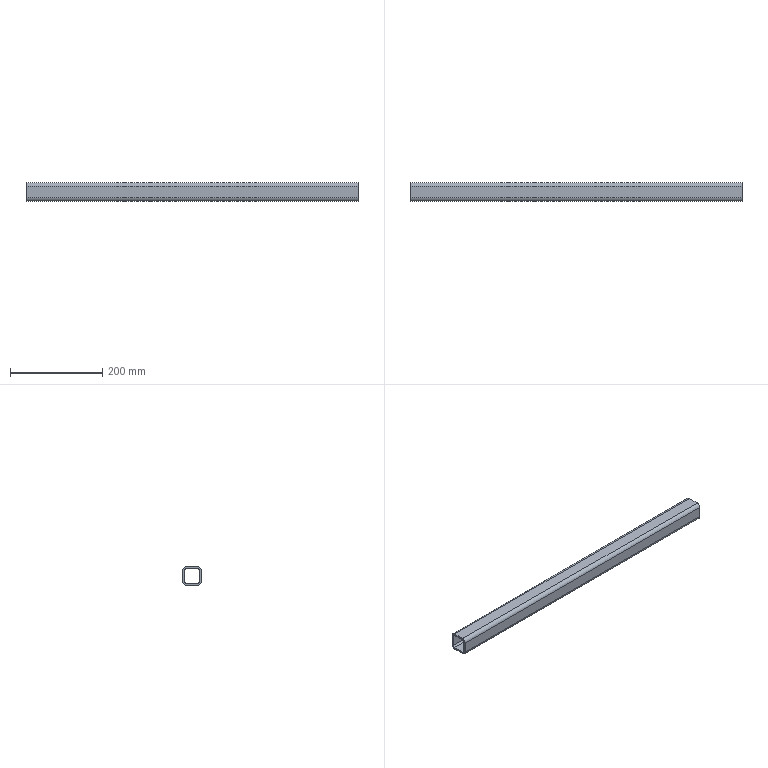Part | SolidWorks | features WeldMemberFeat 1, WeldmentFeature 1 | 1 solid | 18 faces | box 720 x 40 x 40 mm | volume 385053 mm3 | plane 10 | cylinder 8 | commonest cylinder face diameters 8 x4 16 x4
STEP:
#1=CARTESIAN_POINT('',(-1000.,20.,12.));
#2=VERTEX_POINT('',#1);
#3=CARTESIAN_POINT('',(-1000.,12.,20.));
#4=VERTEX_POINT('',#3);
#5=CARTESIAN_POINT('',(-1000.,12.,12.));
#6=DIRECTION('',(1.,0.,0.));
#7=DIRECTION('',(0.,0.,-1.));
#8=AXIS2_PLACEMENT_3D('',#5,#6,#7);
#9=CIRCLE('',#8,8.);
#10=EDGE_CURVE('',#2,#4,#9,.T.);
#11=ORIENTED_EDGE('',*,*,#10,.T.);
#12=CARTESIAN_POINT('',(-280.,12.,20.));
#13=VERTEX_POINT('',#12);
#14=CARTESIAN_POINT('',(-280.,12.,20.));
#15=DIRECTION('',(-1.,0.,0.));
#16=VECTOR('',#15,1000.);
#17=LINE('',#14,#16);
#18=EDGE_CURVE('',#13,#4,#17,.T.);
#19=ORIENTED_EDGE('',*,*,#18,.F.);
#20=CARTESIAN_POINT('',(-280.,20.,12.));
#21=VERTEX_POINT('',#20);
#22=CARTESIAN_POINT('',(-280.,12.,12.));
#23=DIRECTION('',(1.,0.,0.));
#24=DIRECTION('',(0.,0.,-1.));
#25=AXIS2_PLACEMENT_3D('',#22,#23,#24);
#26=CIRCLE('',#25,8.);
#27=EDGE_CURVE('',#21,#13,#26,.T.);
#28=ORIENTED_EDGE('',*,*,#27,.F.);
#29=CARTESIAN_POINT('',(-280.,20.,12.));
#30=DIRECTION('',(-1.,0.,0.));
#31=VECTOR('',#30,1000.);
#32=LINE('',#29,#31);
#33=EDGE_CURVE('',#21,#2,#32,.T.);
#34=ORIENTED_EDGE('',*,*,#33,.T.);
#35=EDGE_LOOP('',(#11,#19,#28,#34));
#36=FACE_OUTER_BOUND('',#35,.T.);
#37=CARTESIAN_POINT('',(-280.,12.,12.));
#38=DIRECTION('',(-1.,0.,0.));
#39=DIRECTION('',(0.,0.,1.));
#40=AXIS2_PLACEMENT_3D('',#37,#38,#39);
#41=CYLINDRICAL_SURFACE('',#40,8.);
#42=ADVANCED_FACE('',(#36),#41,.T.);
#43=CARTESIAN_POINT('',(-1000.,-12.,20.));
#44=VERTEX_POINT('',#43);
#45=CARTESIAN_POINT('',(-1000.,12.,20.));
#46=DIRECTION('',(0.,-1.,0.));
#47=VECTOR('',#46,1000.);
#48=LINE('',#45,#47);
#49=EDGE_CURVE('',#4,#44,#48,.T.);
#50=ORIENTED_EDGE('',*,*,#49,.T.);
#51=CARTESIAN_POINT('',(-280.,-12.,20.));
#52=VERTEX_POINT('',#51);
#53=CARTESIAN_POINT('',(-280.,-12.,20.));
#54=DIRECTION('',(-1.,0.,0.));
#55=VECTOR('',#54,1000.);
#56=LINE('',#53,#55);
#57=EDGE_CURVE('',#52,#44,#56,.T.);
#58=ORIENTED_EDGE('',*,*,#57,.F.);
#59=CARTESIAN_POINT('',(-280.,12.,20.));
#60=DIRECTION('',(0.,-1.,0.));
#61=VECTOR('',#60,1000.);
#62=LINE('',#59,#61);
#63=EDGE_CURVE('',#13,#52,#62,.T.);
#64=ORIENTED_EDGE('',*,*,#63,.F.);
#65=ORIENTED_EDGE('',*,*,#18,.T.);
#66=EDGE_LOOP('',(#50,#58,#64,#65));
#67=FACE_OUTER_BOUND('',#66,.T.);
#68=CARTESIAN_POINT('',(-280.,12.,20.));
#69=DIRECTION('',(0.,0.,-1.));
#70=DIRECTION('',(-1.,0.,0.));
#71=AXIS2_PLACEMENT_3D('',#68,#69,#70);
#72=PLANE('',#71);
#73=ADVANCED_FACE('',(#67),#72,.F.);
#74=CARTESIAN_POINT('',(-1000.,-20.,12.));
#75=VERTEX_POINT('',#74);
#76=CARTESIAN_POINT('',(-1000.,-12.,12.));
#77=DIRECTION('',(1.,0.,0.));
#78=DIRECTION('',(0.,0.,-1.));
#79=AXIS2_PLACEMENT_3D('',#76,#77,#78);
#80=CIRCLE('',#79,8.);
#81=EDGE_CURVE('',#44,#75,#80,.T.);
#82=ORIENTED_EDGE('',*,*,#81,.T.);
#83=CARTESIAN_POINT('',(-280.,-20.,12.));
#84=VERTEX_POINT('',#83);
#85=CARTESIAN_POINT('',(-280.,-20.,12.));
#86=DIRECTION('',(-1.,0.,0.));
#87=VECTOR('',#86,1000.);
#88=LINE('',#85,#87);
#89=EDGE_CURVE('',#84,#75,#88,.T.);
#90=ORIENTED_EDGE('',*,*,#89,.F.);
#91=CARTESIAN_POINT('',(-280.,-12.,12.));
#92=DIRECTION('',(1.,0.,0.));
#93=DIRECTION('',(0.,0.,-1.));
#94=AXIS2_PLACEMENT_3D('',#91,#92,#93);
#95=CIRCLE('',#94,8.);
#96=EDGE_CURVE('',#52,#84,#95,.T.);
#97=ORIENTED_EDGE('',*,*,#96,.F.);
#98=ORIENTED_EDGE('',*,*,#57,.T.);
#99=EDGE_LOOP('',(#82,#90,#97,#98));
#100=FACE_OUTER_BOUND('',#99,.T.);
#101=CARTESIAN_POINT('',(-280.,-12.,12.));
#102=DIRECTION('',(-1.,0.,0.));
#103=DIRECTION('',(0.,0.,1.));
#104=AXIS2_PLACEMENT_3D('',#101,#102,#103);
#105=CYLINDRICAL_SURFACE('',#104,8.);
#106=ADVANCED_FACE('',(#100),#105,.T.);
#107=CARTESIAN_POINT('',(-1000.,-20.,-12.));
#108=VERTEX_POINT('',#107);
#109=CARTESIAN_POINT('',(-1000.,-20.,-12.));
#110=DIRECTION('',(0.,0.,-1.));
#111=VECTOR('',#110,1000.);
#112=LINE('',#109,#111);
#113=EDGE_CURVE('',#75,#108,#112,.T.);
#114=ORIENTED_EDGE('',*,*,#113,.T.);
#115=CARTESIAN_POINT('',(-280.,-20.,-12.));
#116=VERTEX_POINT('',#115);
#117=CARTESIAN_POINT('',(-280.,-20.,-12.));
#118=DIRECTION('',(-1.,0.,0.));
#119=VECTOR('',#118,1000.);
#120=LINE('',#117,#119);
#121=EDGE_CURVE('',#116,#108,#120,.T.);
#122=ORIENTED_EDGE('',*,*,#121,.F.);
#123=CARTESIAN_POINT('',(-280.,-20.,-12.));
#124=DIRECTION('',(0.,0.,-1.));
#125=VECTOR('',#124,1000.);
#126=LINE('',#123,#125);
#127=EDGE_CURVE('',#84,#116,#126,.T.);
#128=ORIENTED_EDGE('',*,*,#127,.F.);
#129=ORIENTED_EDGE('',*,*,#89,.T.);
#130=EDGE_LOOP('',(#114,#122,#128,#129));
#131=FACE_OUTER_BOUND('',#130,.T.);
#132=CARTESIAN_POINT('',(-280.,-20.,-12.));
#133=DIRECTION('',(0.,1.,0.));
#134=DIRECTION('',(0.,0.,1.));
#135=AXIS2_PLACEMENT_3D('',#132,#133,#134);
#136=PLANE('',#135);
#137=ADVANCED_FACE('',(#131),#136,.F.);
#138=CARTESIAN_POINT('',(-1000.,-12.,-20.));
#139=VERTEX_POINT('',#138);
#140=CARTESIAN_POINT('',(-1000.,-12.,-12.));
#141=DIRECTION('',(1.,0.,0.));
#142=DIRECTION('',(0.,0.,-1.));
#143=AXIS2_PLACEMENT_3D('',#140,#141,#142);
#144=CIRCLE('',#143,8.);
#145=EDGE_CURVE('',#108,#139,#144,.T.);
#146=ORIENTED_EDGE('',*,*,#145,.T.);
#147=CARTESIAN_POINT('',(-280.,-12.,-20.));
#148=VERTEX_POINT('',#147);
#149=CARTESIAN_POINT('',(-280.,-12.,-20.));
#150=DIRECTION('',(-1.,0.,0.));
#151=VECTOR('',#150,1000.);
#152=LINE('',#149,#151);
#153=EDGE_CURVE('',#148,#139,#152,.T.);
#154=ORIENTED_EDGE('',*,*,#153,.F.);
#155=CARTESIAN_POINT('',(-280.,-12.,-12.));
#156=DIRECTION('',(1.,0.,0.));
#157=DIRECTION('',(0.,0.,-1.));
#158=AXIS2_PLACEMENT_3D('',#155,#156,#157);
#159=CIRCLE('',#158,8.);
#160=EDGE_CURVE('',#116,#148,#159,.T.);
#161=ORIENTED_EDGE('',*,*,#160,.F.);
#162=ORIENTED_EDGE('',*,*,#121,.T.);
#163=EDGE_LOOP('',(#146,#154,#161,#162));
#164=FACE_OUTER_BOUND('',#163,.T.);
#165=CARTESIAN_POINT('',(-280.,-12.,-12.));
#166=DIRECTION('',(-1.,0.,0.));
#167=DIRECTION('',(0.,0.,1.));
#168=AXIS2_PLACEMENT_3D('',#165,#166,#167);
#169=CYLINDRICAL_SURFACE('',#168,8.);
#170=ADVANCED_FACE('',(#164),#169,.T.);
#171=CARTESIAN_POINT('',(-1000.,12.,-20.));
#172=VERTEX_POINT('',#171);
#173=CARTESIAN_POINT('',(-1000.,-12.,-20.));
#174=DIRECTION('',(0.,1.,0.));
#175=VECTOR('',#174,1000.);
#176=LINE('',#173,#175);
#177=EDGE_CURVE('',#139,#172,#176,.T.);
#178=ORIENTED_EDGE('',*,*,#177,.T.);
#179=CARTESIAN_POINT('',(-280.,12.,-20.));
#180=VERTEX_POINT('',#179);
#181=CARTESIAN_POINT('',(-280.,12.,-20.));
#182=DIRECTION('',(-1.,0.,0.));
#183=VECTOR('',#182,1000.);
#184=LINE('',#181,#183);
#185=EDGE_CURVE('',#180,#172,#184,.T.);
#186=ORIENTED_EDGE('',*,*,#185,.F.);
#187=CARTESIAN_POINT('',(-280.,-12.,-20.));
#188=DIRECTION('',(0.,1.,0.));
#189=VECTOR('',#188,1000.);
#190=LINE('',#187,#189);
#191=EDGE_CURVE('',#148,#180,#190,.T.);
#192=ORIENTED_EDGE('',*,*,#191,.F.);
#193=ORIENTED_EDGE('',*,*,#153,.T.);
#194=EDGE_LOOP('',(#178,#186,#192,#193));
#195=FACE_OUTER_BOUND('',#194,.T.);
#196=CARTESIAN_POINT('',(-280.,-12.,-20.));
#197=DIRECTION('',(0.,0.,1.));
#198=DIRECTION('',(1.,0.,0.));
#199=AXIS2_PLACEMENT_3D('',#196,#197,#198);
#200=PLANE('',#199);
#201=ADVANCED_FACE('',(#195),#200,.F.);
#202=CARTESIAN_POINT('',(-1000.,20.,-12.));
#203=VERTEX_POINT('',#202);
#204=CARTESIAN_POINT('',(-1000.,12.,-12.));
#205=DIRECTION('',(1.,0.,0.));
#206=DIRECTION('',(0.,0.,-1.));
#207=AXIS2_PLACEMENT_3D('',#204,#205,#206);
#208=CIRCLE('',#207,8.);
#209=EDGE_CURVE('',#172,#203,#208,.T.);
#210=ORIENTED_EDGE('',*,*,#209,.T.);
#211=CARTESIAN_POINT('',(-280.,20.,-12.));
#212=VERTEX_POINT('',#211);
#213=CARTESIAN_POINT('',(-280.,20.,-12.));
#214=DIRECTION('',(-1.,0.,0.));
#215=VECTOR('',#214,1000.);
#216=LINE('',#213,#215);
#217=EDGE_CURVE('',#212,#203,#216,.T.);
#218=ORIENTED_EDGE('',*,*,#217,.F.);
#219=CARTESIAN_POINT('',(-280.,12.,-12.));
#220=DIRECTION('',(1.,0.,0.));
#221=DIRECTION('',(0.,0.,-1.));
#222=AXIS2_PLACEMENT_3D('',#219,#220,#221);
#223=CIRCLE('',#222,8.);
#224=EDGE_CURVE('',#180,#212,#223,.T.);
#225=ORIENTED_EDGE('',*,*,#224,.F.);
#226=ORIENTED_EDGE('',*,*,#185,.T.);
#227=EDGE_LOOP('',(#210,#218,#225,#226));
#228=FACE_OUTER_BOUND('',#227,.T.);
#229=CARTESIAN_POINT('',(-280.,12.,-12.));
#230=DIRECTION('',(-1.,0.,0.));
#231=DIRECTION('',(0.,0.,1.));
#232=AXIS2_PLACEMENT_3D('',#229,#230,#231);
#233=CYLINDRICAL_SURFACE('',#232,8.);
#234=ADVANCED_FACE('',(#228),#233,.T.);
#235=CARTESIAN_POINT('',(-1000.,-12.,16.));
#236=VERTEX_POINT('',#235);
#237=CARTESIAN_POINT('',(-1000.,-16.,12.));
#238=VERTEX_POINT('',#237);
#239=CARTESIAN_POINT('',(-1000.,-12.,12.));
#240=DIRECTION('',(1.,0.,0.));
#241=DIRECTION('',(0.,0.,-1.));
#242=AXIS2_PLACEMENT_3D('',#239,#240,#241);
#243=CIRCLE('',#242,4.);
#244=EDGE_CURVE('',#236,#238,#243,.T.);
#245=ORIENTED_EDGE('',*,*,#244,.F.);
#246=CARTESIAN_POINT('',(-280.,-12.,16.));
#247=VERTEX_POINT('',#246);
#248=CARTESIAN_POINT('',(-280.,-12.,16.));
#249=DIRECTION('',(-1.,0.,0.));
#250=VECTOR('',#249,1000.);
#251=LINE('',#248,#250);
#252=EDGE_CURVE('',#247,#236,#251,.T.);
#253=ORIENTED_EDGE('',*,*,#252,.F.);
#254=CARTESIAN_POINT('',(-280.,-16.,12.));
#255=VERTEX_POINT('',#254);
#256=CARTESIAN_POINT('',(-280.,-12.,12.));
#257=DIRECTION('',(1.,0.,0.));
#258=DIRECTION('',(0.,0.,-1.));
#259=AXIS2_PLACEMENT_3D('',#256,#257,#258);
#260=CIRCLE('',#259,4.);
#261=EDGE_CURVE('',#247,#255,#260,.T.);
#262=ORIENTED_EDGE('',*,*,#261,.T.);
#263=CARTESIAN_POINT('',(-280.,-16.,12.));
#264=DIRECTION('',(-1.,0.,0.));
#265=VECTOR('',#264,1000.);
#266=LINE('',#263,#265);
#267=EDGE_CURVE('',#255,#238,#266,.T.);
#268=ORIENTED_EDGE('',*,*,#267,.T.);
#269=EDGE_LOOP('',(#245,#253,#262,#268));
#270=FACE_OUTER_BOUND('',#269,.T.);
#271=CARTESIAN_POINT('',(-280.,-12.,12.));
#272=DIRECTION('',(-1.,0.,0.));
#273=DIRECTION('',(0.,0.,1.));
#274=AXIS2_PLACEMENT_3D('',#271,#272,#273);
#275=CYLINDRICAL_SURFACE('',#274,4.);
#276=ADVANCED_FACE('',(#270),#275,.F.);
#277=CARTESIAN_POINT('',(-1000.,12.,16.));
#278=VERTEX_POINT('',#277);
#279=CARTESIAN_POINT('',(-1000.,12.,16.));
#280=DIRECTION('',(0.,-1.,0.));
#281=VECTOR('',#280,1000.);
#282=LINE('',#279,#281);
#283=EDGE_CURVE('',#278,#236,#282,.T.);
#284=ORIENTED_EDGE('',*,*,#283,.F.);
#285=CARTESIAN_POINT('',(-280.,12.,16.));
#286=VERTEX_POINT('',#285);
#287=CARTESIAN_POINT('',(-280.,12.,16.));
#288=DIRECTION('',(-1.,0.,0.));
#289=VECTOR('',#288,1000.);
#290=LINE('',#287,#289);
#291=EDGE_CURVE('',#286,#278,#290,.T.);
#292=ORIENTED_EDGE('',*,*,#291,.F.);
#293=CARTESIAN_POINT('',(-280.,12.,16.));
#294=DIRECTION('',(0.,-1.,0.));
#295=VECTOR('',#294,1000.);
#296=LINE('',#293,#295);
#297=EDGE_CURVE('',#286,#247,#296,.T.);
#298=ORIENTED_EDGE('',*,*,#297,.T.);
#299=ORIENTED_EDGE('',*,*,#252,.T.);
#300=EDGE_LOOP('',(#284,#292,#298,#299));
#301=FACE_OUTER_BOUND('',#300,.T.);
#302=CARTESIAN_POINT('',(-280.,12.,16.));
#303=DIRECTION('',(0.,0.,-1.));
#304=DIRECTION('',(-1.,0.,0.));
#305=AXIS2_PLACEMENT_3D('',#302,#303,#304);
#306=PLANE('',#305);
#307=ADVANCED_FACE('',(#301),#306,.T.);
#308=CARTESIAN_POINT('',(-1000.,16.,12.));
#309=VERTEX_POINT('',#308);
#310=CARTESIAN_POINT('',(-1000.,12.,12.));
#311=DIRECTION('',(1.,0.,0.));
#312=DIRECTION('',(0.,0.,-1.));
#313=AXIS2_PLACEMENT_3D('',#310,#311,#312);
#314=CIRCLE('',#313,4.);
#315=EDGE_CURVE('',#309,#278,#314,.T.);
#316=ORIENTED_EDGE('',*,*,#315,.F.);
#317=CARTESIAN_POINT('',(-280.,16.,12.));
#318=VERTEX_POINT('',#317);
#319=CARTESIAN_POINT('',(-280.,16.,12.));
#320=DIRECTION('',(-1.,0.,0.));
#321=VECTOR('',#320,1000.);
#322=LINE('',#319,#321);
#323=EDGE_CURVE('',#318,#309,#322,.T.);
#324=ORIENTED_EDGE('',*,*,#323,.F.);
#325=CARTESIAN_POINT('',(-280.,12.,12.));
#326=DIRECTION('',(1.,0.,0.));
#327=DIRECTION('',(0.,0.,-1.));
#328=AXIS2_PLACEMENT_3D('',#325,#326,#327);
#329=CIRCLE('',#328,4.);
#330=EDGE_CURVE('',#318,#286,#329,.T.);
#331=ORIENTED_EDGE('',*,*,#330,.T.);
#332=ORIENTED_EDGE('',*,*,#291,.T.);
#333=EDGE_LOOP('',(#316,#324,#331,#332));
#334=FACE_OUTER_BOUND('',#333,.T.);
#335=CARTESIAN_POINT('',(-280.,12.,12.));
#336=DIRECTION('',(-1.,0.,0.));
#337=DIRECTION('',(0.,0.,1.));
#338=AXIS2_PLACEMENT_3D('',#335,#336,#337);
#339=CYLINDRICAL_SURFACE('',#338,4.);
#340=ADVANCED_FACE('',(#334),#339,.F.);
#341=CARTESIAN_POINT('',(-1000.,16.,-12.));
#342=VERTEX_POINT('',#341);
#343=CARTESIAN_POINT('',(-1000.,16.,12.));
#344=DIRECTION('',(0.,0.,1.));
#345=VECTOR('',#344,1000.);
#346=LINE('',#343,#345);
#347=EDGE_CURVE('',#342,#309,#346,.T.);
#348=ORIENTED_EDGE('',*,*,#347,.F.);
#349=CARTESIAN_POINT('',(-280.,16.,-12.));
#350=VERTEX_POINT('',#349);
#351=CARTESIAN_POINT('',(-280.,16.,-12.));
#352=DIRECTION('',(-1.,0.,0.));
#353=VECTOR('',#352,1000.);
#354=LINE('',#351,#353);
#355=EDGE_CURVE('',#350,#342,#354,.T.);
#356=ORIENTED_EDGE('',*,*,#355,.F.);
#357=CARTESIAN_POINT('',(-280.,16.,12.));
#358=DIRECTION('',(0.,0.,1.));
#359=VECTOR('',#358,1000.);
#360=LINE('',#357,#359);
#361=EDGE_CURVE('',#350,#318,#360,.T.);
#362=ORIENTED_EDGE('',*,*,#361,.T.);
#363=ORIENTED_EDGE('',*,*,#323,.T.);
#364=EDGE_LOOP('',(#348,#356,#362,#363));
#365=FACE_OUTER_BOUND('',#364,.T.);
#366=CARTESIAN_POINT('',(-280.,16.,12.));
#367=DIRECTION('',(0.,-1.,0.));
#368=DIRECTION('',(0.,0.,-1.));
#369=AXIS2_PLACEMENT_3D('',#366,#367,#368);
#370=PLANE('',#369);
#371=ADVANCED_FACE('',(#365),#370,.T.);
#372=CARTESIAN_POINT('',(-1000.,12.,-16.));
#373=VERTEX_POINT('',#372);
#374=CARTESIAN_POINT('',(-1000.,12.,-12.));
#375=DIRECTION('',(1.,0.,0.));
#376=DIRECTION('',(0.,0.,-1.));
#377=AXIS2_PLACEMENT_3D('',#374,#375,#376);
#378=CIRCLE('',#377,4.);
#379=EDGE_CURVE('',#373,#342,#378,.T.);
#380=ORIENTED_EDGE('',*,*,#379,.F.);
#381=CARTESIAN_POINT('',(-280.,12.,-16.));
#382=VERTEX_POINT('',#381);
#383=CARTESIAN_POINT('',(-280.,12.,-16.));
#384=DIRECTION('',(-1.,0.,0.));
#385=VECTOR('',#384,1000.);
#386=LINE('',#383,#385);
#387=EDGE_CURVE('',#382,#373,#386,.T.);
#388=ORIENTED_EDGE('',*,*,#387,.F.);
#389=CARTESIAN_POINT('',(-280.,12.,-12.));
#390=DIRECTION('',(1.,0.,0.));
#391=DIRECTION('',(0.,0.,-1.));
#392=AXIS2_PLACEMENT_3D('',#389,#390,#391);
#393=CIRCLE('',#392,4.);
#394=EDGE_CURVE('',#382,#350,#393,.T.);
#395=ORIENTED_EDGE('',*,*,#394,.T.);
#396=ORIENTED_EDGE('',*,*,#355,.T.);
#397=EDGE_LOOP('',(#380,#388,#395,#396));
#398=FACE_OUTER_BOUND('',#397,.T.);
#399=CARTESIAN_POINT('',(-280.,12.,-12.));
#400=DIRECTION('',(-1.,0.,0.));
#401=DIRECTION('',(0.,0.,1.));
#402=AXIS2_PLACEMENT_3D('',#399,#400,#401);
#403=CYLINDRICAL_SURFACE('',#402,4.);
#404=ADVANCED_FACE('',(#398),#403,.F.);
#405=CARTESIAN_POINT('',(-1000.,-12.,-16.));
#406=VERTEX_POINT('',#405);
#407=CARTESIAN_POINT('',(-1000.,-12.,-16.));
#408=DIRECTION('',(0.,1.,0.));
#409=VECTOR('',#408,1000.);
#410=LINE('',#407,#409);
#411=EDGE_CURVE('',#406,#373,#410,.T.);
#412=ORIENTED_EDGE('',*,*,#411,.F.);
#413=CARTESIAN_POINT('',(-280.,-12.,-16.));
#414=VERTEX_POINT('',#413);
#415=CARTESIAN_POINT('',(-280.,-12.,-16.));
#416=DIRECTION('',(-1.,0.,0.));
#417=VECTOR('',#416,1000.);
#418=LINE('',#415,#417);
#419=EDGE_CURVE('',#414,#406,#418,.T.);
#420=ORIENTED_EDGE('',*,*,#419,.F.);
#421=CARTESIAN_POINT('',(-280.,-12.,-16.));
#422=DIRECTION('',(0.,1.,0.));
#423=VECTOR('',#422,1000.);
#424=LINE('',#421,#423);
#425=EDGE_CURVE('',#414,#382,#424,.T.);
#426=ORIENTED_EDGE('',*,*,#425,.T.);
#427=ORIENTED_EDGE('',*,*,#387,.T.);
#428=EDGE_LOOP('',(#412,#420,#426,#427));
#429=FACE_OUTER_BOUND('',#428,.T.);
#430=CARTESIAN_POINT('',(-280.,-12.,-16.));
#431=DIRECTION('',(0.,0.,1.));
#432=DIRECTION('',(1.,0.,0.));
#433=AXIS2_PLACEMENT_3D('',#430,#431,#432);
#434=PLANE('',#433);
#435=ADVANCED_FACE('',(#429),#434,.T.);
#436=CARTESIAN_POINT('',(-1000.,-16.,-12.));
#437=VERTEX_POINT('',#436);
#438=CARTESIAN_POINT('',(-1000.,-12.,-12.));
#439=DIRECTION('',(1.,0.,0.));
#440=DIRECTION('',(0.,0.,-1.));
#441=AXIS2_PLACEMENT_3D('',#438,#439,#440);
#442=CIRCLE('',#441,4.);
#443=EDGE_CURVE('',#437,#406,#442,.T.);
#444=ORIENTED_EDGE('',*,*,#443,.F.);
#445=CARTESIAN_POINT('',(-280.,-16.,-12.));
#446=VERTEX_POINT('',#445);
#447=CARTESIAN_POINT('',(-280.,-16.,-12.));
#448=DIRECTION('',(-1.,0.,0.));
#449=VECTOR('',#448,1000.);
#450=LINE('',#447,#449);
#451=EDGE_CURVE('',#446,#437,#450,.T.);
#452=ORIENTED_EDGE('',*,*,#451,.F.);
#453=CARTESIAN_POINT('',(-280.,-12.,-12.));
#454=DIRECTION('',(1.,0.,0.));
#455=DIRECTION('',(0.,0.,-1.));
#456=AXIS2_PLACEMENT_3D('',#453,#454,#455);
#457=CIRCLE('',#456,4.);
#458=EDGE_CURVE('',#446,#414,#457,.T.);
#459=ORIENTED_EDGE('',*,*,#458,.T.);
#460=ORIENTED_EDGE('',*,*,#419,.T.);
#461=EDGE_LOOP('',(#444,#452,#459,#460));
#462=FACE_OUTER_BOUND('',#461,.T.);
#463=CARTESIAN_POINT('',(-280.,-12.,-12.));
#464=DIRECTION('',(-1.,0.,0.));
#465=DIRECTION('',(0.,0.,1.));
#466=AXIS2_PLACEMENT_3D('',#463,#464,#465);
#467=CYLINDRICAL_SURFACE('',#466,4.);
#468=ADVANCED_FACE('',(#462),#467,.F.);
#469=CARTESIAN_POINT('',(-1000.,-16.,-12.));
#470=DIRECTION('',(0.,0.,-1.));
#471=VECTOR('',#470,1000.);
#472=LINE('',#469,#471);
#473=EDGE_CURVE('',#238,#437,#472,.T.);
#474=ORIENTED_EDGE('',*,*,#473,.F.);
#475=ORIENTED_EDGE('',*,*,#267,.F.);
#476=CARTESIAN_POINT('',(-280.,-16.,-12.));
#477=DIRECTION('',(0.,0.,-1.));
#478=VECTOR('',#477,1000.);
#479=LINE('',#476,#478);
#480=EDGE_CURVE('',#255,#446,#479,.T.);
#481=ORIENTED_EDGE('',*,*,#480,.T.);
#482=ORIENTED_EDGE('',*,*,#451,.T.);
#483=EDGE_LOOP('',(#474,#475,#481,#482));
#484=FACE_OUTER_BOUND('',#483,.T.);
#485=CARTESIAN_POINT('',(-280.,-16.,-12.));
#486=DIRECTION('',(0.,1.,0.));
#487=DIRECTION('',(0.,0.,1.));
#488=AXIS2_PLACEMENT_3D('',#485,#486,#487);
#489=PLANE('',#488);
#490=ADVANCED_FACE('',(#484),#489,.T.);
#491=CARTESIAN_POINT('',(-1000.,20.,12.));
#492=DIRECTION('',(0.,0.,1.));
#493=VECTOR('',#492,1000.);
#494=LINE('',#491,#493);
#495=EDGE_CURVE('',#203,#2,#494,.T.);
#496=ORIENTED_EDGE('',*,*,#495,.T.);
#497=ORIENTED_EDGE('',*,*,#33,.F.);
#498=CARTESIAN_POINT('',(-280.,20.,12.));
#499=DIRECTION('',(0.,0.,1.));
#500=VECTOR('',#499,1000.);
#501=LINE('',#498,#500);
#502=EDGE_CURVE('',#212,#21,#501,.T.);
#503=ORIENTED_EDGE('',*,*,#502,.F.);
#504=ORIENTED_EDGE('',*,*,#217,.T.);
#505=EDGE_LOOP('',(#496,#497,#503,#504));
#506=FACE_OUTER_BOUND('',#505,.T.);
#507=CARTESIAN_POINT('',(-280.,20.,12.));
#508=DIRECTION('',(0.,-1.,0.));
#509=DIRECTION('',(0.,0.,-1.));
#510=AXIS2_PLACEMENT_3D('',#507,#508,#509);
#511=PLANE('',#510);
#512=ADVANCED_FACE('',(#506),#511,.F.);
#513=ORIENTED_EDGE('',*,*,#261,.F.);
#514=ORIENTED_EDGE('',*,*,#297,.F.);
#515=ORIENTED_EDGE('',*,*,#330,.F.);
#516=ORIENTED_EDGE('',*,*,#361,.F.);
#517=ORIENTED_EDGE('',*,*,#394,.F.);
#518=ORIENTED_EDGE('',*,*,#425,.F.);
#519=ORIENTED_EDGE('',*,*,#458,.F.);
#520=ORIENTED_EDGE('',*,*,#480,.F.);
#521=EDGE_LOOP('',(#513,#514,#515,#516,#517,#518,#519,#520));
#522=FACE_BOUND('',#521,.T.);
#523=ORIENTED_EDGE('',*,*,#27,.T.);
#524=ORIENTED_EDGE('',*,*,#63,.T.);
#525=ORIENTED_EDGE('',*,*,#96,.T.);
#526=ORIENTED_EDGE('',*,*,#127,.T.);
#527=ORIENTED_EDGE('',*,*,#160,.T.);
#528=ORIENTED_EDGE('',*,*,#191,.T.);
#529=ORIENTED_EDGE('',*,*,#224,.T.);
#530=ORIENTED_EDGE('',*,*,#502,.T.);
#531=EDGE_LOOP('',(#523,#524,#525,#526,#527,#528,#529,#530));
#532=FACE_OUTER_BOUND('',#531,.T.);
#533=CARTESIAN_POINT('',(-280.,12.,12.));
#534=DIRECTION('',(1.,0.,0.));
#535=DIRECTION('',(0.,0.,-1.));
#536=AXIS2_PLACEMENT_3D('',#533,#534,#535);
#537=PLANE('',#536);
#538=ADVANCED_FACE('',(#522,#532),#537,.T.);
#539=ORIENTED_EDGE('',*,*,#244,.T.);
#540=ORIENTED_EDGE('',*,*,#473,.T.);
#541=ORIENTED_EDGE('',*,*,#443,.T.);
#542=ORIENTED_EDGE('',*,*,#411,.T.);
#543=ORIENTED_EDGE('',*,*,#379,.T.);
#544=ORIENTED_EDGE('',*,*,#347,.T.);
#545=ORIENTED_EDGE('',*,*,#315,.T.);
#546=ORIENTED_EDGE('',*,*,#283,.T.);
#547=EDGE_LOOP('',(#539,#540,#541,#542,#543,#544,#545,#546));
#548=FACE_BOUND('',#547,.T.);
#549=ORIENTED_EDGE('',*,*,#10,.F.);
#550=ORIENTED_EDGE('',*,*,#495,.F.);
#551=ORIENTED_EDGE('',*,*,#209,.F.);
#552=ORIENTED_EDGE('',*,*,#177,.F.);
#553=ORIENTED_EDGE('',*,*,#145,.F.);
#554=ORIENTED_EDGE('',*,*,#113,.F.);
#555=ORIENTED_EDGE('',*,*,#81,.F.);
#556=ORIENTED_EDGE('',*,*,#49,.F.);
#557=EDGE_LOOP('',(#549,#550,#551,#552,#553,#554,#555,#556));
#558=FACE_OUTER_BOUND('',#557,.T.);
#559=CARTESIAN_POINT('',(-1000.,12.,12.));
#560=DIRECTION('',(1.,0.,0.));
#561=DIRECTION('',(0.,0.,-1.));
#562=AXIS2_PLACEMENT_3D('',#559,#560,#561);
#563=PLANE('',#562);
#564=ADVANCED_FACE('',(#548,#558),#563,.F.);
#565=CLOSED_SHELL('',(#42,#73,#106,#137,#170,#201,#234,#276,#307,#340,#371,#404,#435,#468,#490,#512,#538,#564));
#566=MANIFOLD_SOLID_BREP('',#565);
#567=CARTESIAN_POINT('',(0.,0.,0.));
#568=DIRECTION('',(0.,0.,1.));
#569=DIRECTION('',(1.,0.,0.));
#570=AXIS2_PLACEMENT_3D('',#567,#568,#569);
#571=(LENGTH_UNIT()NAMED_UNIT(*)SI_UNIT(.MILLI.,.METRE.));
#572=UNCERTAINTY_MEASURE_WITH_UNIT(LENGTH_MEASURE(0.00001),#571,'','');
#573=(NAMED_UNIT(*)PLANE_ANGLE_UNIT()SI_UNIT($,.RADIAN.));
#574=(NAMED_UNIT(*)SI_UNIT($,.STERADIAN.)SOLID_ANGLE_UNIT());
#575=(GEOMETRIC_REPRESENTATION_CONTEXT(3)GLOBAL_UNCERTAINTY_ASSIGNED_CONTEXT((#572))GLOBAL_UNIT_ASSIGNED_CONTEXT((#571,#573,#574))REPRESENTATION_CONTEXT('',''));
#576=ADVANCED_BREP_SHAPE_REPRESENTATION('',(#566,#570),#575);